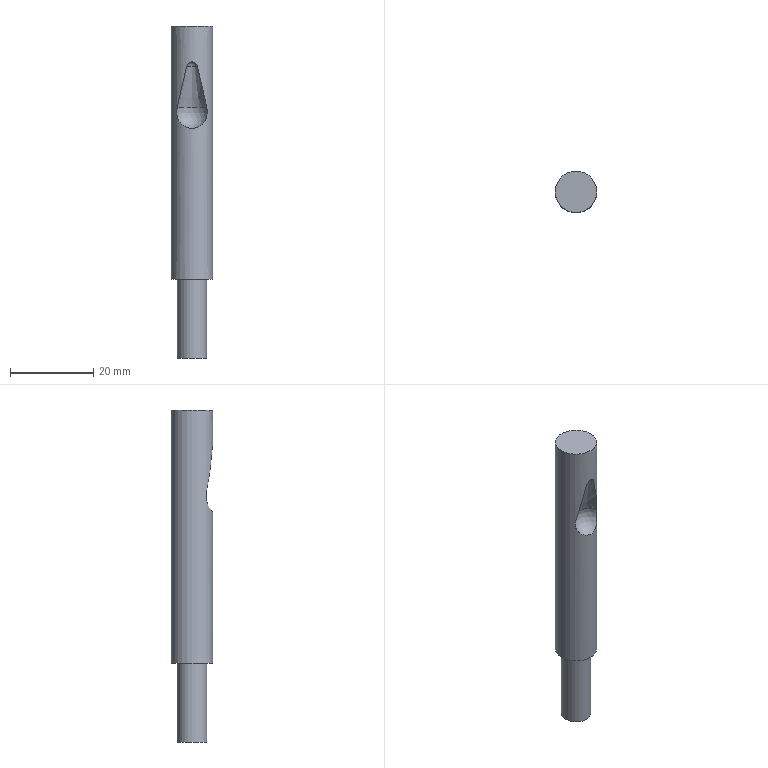Part | NX | features solid 2 | 1 solid | 8 faces | volume 5366 mm3 | plane 3 | cylinder 2 | sphere 2 | cone 1 | commonest cylinder face diameters 7.1 x1 10 x1
STEP:
#1=CARTESIAN_POINT('',(-337.549,205.711,111.333));
#2=VERTEX_POINT('',#1);
#3=CARTESIAN_POINT('',(-335.258,204.378,121.333));
#4=VERTEX_POINT('',#3);
#5=CARTESIAN_POINT('',(-337.549,205.711,111.333));
#6=CARTESIAN_POINT('',(-336.897,205.046,114.658));
#7=CARTESIAN_POINT('',(-336.099,204.6,117.992));
#8=CARTESIAN_POINT('',(-335.258,204.378,121.333));
#9=B_SPLINE_CURVE_WITH_KNOTS('',3,(#5,#6,#7,#8),.UNSPECIFIED.,.F.,.F.,(4,4),(0.000000207,0.01035),.UNSPECIFIED.);
#10=EDGE_CURVE('',#2,#4,#9,.T.);
#11=ORIENTED_EDGE('',*,*,#10,.T.);
#12=CARTESIAN_POINT('',(-332.698,204.378,121.333));
#13=VERTEX_POINT('',#12);
#14=CARTESIAN_POINT('',(-335.258,204.378,121.333));
#15=CARTESIAN_POINT('',(-335.114,204.339,121.906));
#16=CARTESIAN_POINT('',(-333.98,204.083,122.76));
#17=CARTESIAN_POINT('',(-332.842,204.339,121.906));
#18=CARTESIAN_POINT('',(-332.698,204.378,121.333));
#19=B_SPLINE_CURVE_WITH_KNOTS('',3,(#14,#15,#16,#17,#18),.UNSPECIFIED.,.F.,.F.,(4,1,4),(0.000000204,0.001751,0.003502),.UNSPECIFIED.);
#20=EDGE_CURVE('',#4,#13,#19,.T.);
#21=ORIENTED_EDGE('',*,*,#20,.T.);
#22=CARTESIAN_POINT('',(-330.407,205.711,111.333));
#23=VERTEX_POINT('',#22);
#24=CARTESIAN_POINT('',(-332.698,204.378,121.333));
#25=CARTESIAN_POINT('',(-331.856,204.6,117.991));
#26=CARTESIAN_POINT('',(-331.059,205.046,114.66));
#27=CARTESIAN_POINT('',(-330.407,205.711,111.333));
#28=B_SPLINE_CURVE_WITH_KNOTS('',3,(#24,#25,#26,#27),.UNSPECIFIED.,.F.,.F.,(4,4),(0.000000207,0.01036),.UNSPECIFIED.);
#29=EDGE_CURVE('',#13,#23,#28,.T.);
#30=ORIENTED_EDGE('',*,*,#29,.T.);
#31=CARTESIAN_POINT('',(-330.407,205.711,111.333));
#32=CARTESIAN_POINT('',(-330.29,205.83,110.737));
#33=CARTESIAN_POINT('',(-330.271,205.852,109.48));
#34=CARTESIAN_POINT('',(-330.868,205.236,107.792));
#35=CARTESIAN_POINT('',(-332.143,204.456,106.625));
#36=CARTESIAN_POINT('',(-333.967,204.089,106.188));
#37=CARTESIAN_POINT('',(-335.81,204.453,106.621));
#38=CARTESIAN_POINT('',(-337.087,205.236,107.792));
#39=CARTESIAN_POINT('',(-337.684,205.851,109.477));
#40=CARTESIAN_POINT('',(-337.666,205.83,110.737));
#41=CARTESIAN_POINT('',(-337.549,205.711,111.333));
#42=B_SPLINE_CURVE_WITH_KNOTS('',3,(#31,#32,#33,#34,#35,#36,#37,#38,#39,#40,#41),.UNSPECIFIED.,.F.,.F.,(4,1,1,1,1,1,1,1,4),(0.000000205,0.001831,0.003662,0.005493,0.007324,0.009155,0.01099,0.01282,0.01465),.UNSPECIFIED.);
#43=EDGE_CURVE('',#23,#2,#42,.T.);
#44=ORIENTED_EDGE('',*,*,#43,.T.);
#45=EDGE_LOOP('',(#11,#21,#30,#44));
#46=FACE_BOUND('',#45,.T.);
#47=CARTESIAN_POINT('',(-338.978,209.211,131.));
#48=VERTEX_POINT('',#47);
#49=CARTESIAN_POINT('',(-333.978,209.211,131.));
#50=DIRECTION('',(0.,0.,1.));
#51=DIRECTION('',(-1.,0.,0.));
#52=AXIS2_PLACEMENT_3D('',#49,#50,#51);
#53=CIRCLE('',#52,5.);
#54=EDGE_CURVE('',#48,#48,#53,.T.);
#55=ORIENTED_EDGE('',*,*,#54,.F.);
#56=EDGE_LOOP('',(#55));
#57=FACE_BOUND('',#56,.T.);
#58=CARTESIAN_POINT('',(-338.978,209.211,70.));
#59=VERTEX_POINT('',#58);
#60=CARTESIAN_POINT('',(-333.978,209.211,70.));
#61=DIRECTION('',(0.,0.,1.));
#62=DIRECTION('',(-1.,0.,0.));
#63=AXIS2_PLACEMENT_3D('',#60,#61,#62);
#64=CIRCLE('',#63,5.);
#65=EDGE_CURVE('',#59,#59,#64,.T.);
#66=ORIENTED_EDGE('',*,*,#65,.T.);
#67=EDGE_LOOP('',(#66));
#68=FACE_BOUND('',#67,.T.);
#69=CARTESIAN_POINT('',(-333.978,209.211,131.));
#70=DIRECTION('',(0.,0.,-1.));
#71=DIRECTION('',(1.,0.,0.));
#72=AXIS2_PLACEMENT_3D('',#69,#70,#71);
#73=CYLINDRICAL_SURFACE('',#72,5.);
#74=ADVANCED_FACE('',(#46,#57,#68),#73,.T.);
#75=ORIENTED_EDGE('',*,*,#54,.T.);
#76=EDGE_LOOP('',(#75));
#77=FACE_BOUND('',#76,.T.);
#78=CARTESIAN_POINT('',(-333.978,209.211,131.));
#79=DIRECTION('',(0.,0.,1.));
#80=DIRECTION('',(-1.,0.,0.));
#81=AXIS2_PLACEMENT_3D('',#78,#79,#80);
#82=PLANE('',#81);
#83=ADVANCED_FACE('',(#77),#82,.T.);
#84=CARTESIAN_POINT('',(-337.528,209.211,70.));
#85=VERTEX_POINT('',#84);
#86=CARTESIAN_POINT('',(-333.978,209.211,70.));
#87=DIRECTION('',(0.,0.,1.));
#88=DIRECTION('',(-1.,0.,0.));
#89=AXIS2_PLACEMENT_3D('',#86,#87,#88);
#90=CIRCLE('',#89,3.55);
#91=EDGE_CURVE('',#85,#85,#90,.T.);
#92=ORIENTED_EDGE('',*,*,#91,.T.);
#93=EDGE_LOOP('',(#92));
#94=FACE_BOUND('',#93,.T.);
#95=ORIENTED_EDGE('',*,*,#65,.F.);
#96=EDGE_LOOP('',(#95));
#97=FACE_BOUND('',#96,.T.);
#98=CARTESIAN_POINT('',(-333.978,209.211,70.));
#99=DIRECTION('',(0.,0.,1.));
#100=DIRECTION('',(-1.,0.,0.));
#101=AXIS2_PLACEMENT_3D('',#98,#99,#100);
#102=PLANE('',#101);
#103=ADVANCED_FACE('',(#94,#97),#102,.F.);
#104=CARTESIAN_POINT('',(-337.528,209.211,51.));
#105=VERTEX_POINT('',#104);
#106=CARTESIAN_POINT('',(-333.978,209.211,51.));
#107=DIRECTION('',(0.,0.,1.));
#108=DIRECTION('',(-1.,0.,0.));
#109=AXIS2_PLACEMENT_3D('',#106,#107,#108);
#110=CIRCLE('',#109,3.55);
#111=EDGE_CURVE('',#105,#105,#110,.T.);
#112=ORIENTED_EDGE('',*,*,#111,.T.);
#113=EDGE_LOOP('',(#112));
#114=FACE_BOUND('',#113,.T.);
#115=ORIENTED_EDGE('',*,*,#91,.F.);
#116=EDGE_LOOP('',(#115));
#117=FACE_BOUND('',#116,.T.);
#118=CARTESIAN_POINT('',(-333.978,209.211,51.));
#119=DIRECTION('',(0.,0.,1.));
#120=DIRECTION('',(-1.,0.,0.));
#121=AXIS2_PLACEMENT_3D('',#118,#119,#120);
#122=CYLINDRICAL_SURFACE('',#121,3.55);
#123=ADVANCED_FACE('',(#114,#117),#122,.T.);
#124=ORIENTED_EDGE('',*,*,#111,.F.);
#125=EDGE_LOOP('',(#124));
#126=FACE_BOUND('',#125,.T.);
#127=CARTESIAN_POINT('',(-333.978,209.211,51.));
#128=DIRECTION('',(0.,0.,1.));
#129=DIRECTION('',(-1.,0.,0.));
#130=AXIS2_PLACEMENT_3D('',#127,#128,#129);
#131=PLANE('',#130);
#132=ADVANCED_FACE('',(#126),#131,.F.);
#133=CARTESIAN_POINT('',(-333.978,204.211,111.333));
#134=DIRECTION('',(0.,0.,-1.));
#135=DIRECTION('',(1.,0.,0.));
#136=AXIS2_PLACEMENT_3D('',#133,#134,#135);
#137=CIRCLE('',#136,3.873);
#138=EDGE_CURVE('',#2,#23,#137,.T.);
#139=ORIENTED_EDGE('',*,*,#138,.F.);
#140=ORIENTED_EDGE('',*,*,#43,.F.);
#141=EDGE_LOOP('',(#139,#140));
#142=FACE_BOUND('',#141,.T.);
#143=CARTESIAN_POINT('',(-333.978,204.211,110.333));
#144=DIRECTION('',(0.,0.,-1.));
#145=DIRECTION('',(1.,0.,0.));
#146=AXIS2_PLACEMENT_3D('',#143,#144,#145);
#147=SPHERICAL_SURFACE('',#146,4.);
#148=ADVANCED_FACE('',(#142),#147,.F.);
#149=CARTESIAN_POINT('',(-333.978,204.211,121.333));
#150=DIRECTION('',(0.,0.,-1.));
#151=DIRECTION('',(1.,0.,0.));
#152=AXIS2_PLACEMENT_3D('',#149,#150,#151);
#153=CIRCLE('',#152,1.291);
#154=EDGE_CURVE('',#4,#13,#153,.T.);
#155=ORIENTED_EDGE('',*,*,#154,.F.);
#156=ORIENTED_EDGE('',*,*,#10,.F.);
#157=ORIENTED_EDGE('',*,*,#138,.T.);
#158=ORIENTED_EDGE('',*,*,#29,.F.);
#159=EDGE_LOOP('',(#155,#156,#157,#158));
#160=FACE_BOUND('',#159,.T.);
#161=CARTESIAN_POINT('',(-333.978,204.211,111.333));
#162=DIRECTION('',(0.,0.,-1.));
#163=DIRECTION('',(1.,0.,0.));
#164=AXIS2_PLACEMENT_3D('',#161,#162,#163);
#165=CONICAL_SURFACE('',#164,3.873,0.2527);
#166=ADVANCED_FACE('',(#160),#165,.F.);
#167=ORIENTED_EDGE('',*,*,#154,.T.);
#168=ORIENTED_EDGE('',*,*,#20,.F.);
#169=EDGE_LOOP('',(#167,#168));
#170=FACE_BOUND('',#169,.T.);
#171=CARTESIAN_POINT('',(-333.978,204.211,121.));
#172=DIRECTION('',(0.,0.,-1.));
#173=DIRECTION('',(-1.,0.,0.));
#174=AXIS2_PLACEMENT_3D('',#171,#172,#173);
#175=SPHERICAL_SURFACE('',#174,1.333);
#176=ADVANCED_FACE('',(#170),#175,.F.);
#177=CLOSED_SHELL('',(#74,#83,#103,#123,#132,#148,#166,#176));
#178=MANIFOLD_SOLID_BREP('',#177);
#179=(LENGTH_UNIT()NAMED_UNIT(*)SI_UNIT(.MILLI.,.METRE.));
#180=UNCERTAINTY_MEASURE_WITH_UNIT(LENGTH_MEASURE(0.0508),#179,'','');
#181=(NAMED_UNIT(*)PLANE_ANGLE_UNIT()SI_UNIT($,.RADIAN.));
#182=(NAMED_UNIT(*)SI_UNIT($,.STERADIAN.)SOLID_ANGLE_UNIT());
#183=(GEOMETRIC_REPRESENTATION_CONTEXT(3)GLOBAL_UNCERTAINTY_ASSIGNED_CONTEXT((#180))GLOBAL_UNIT_ASSIGNED_CONTEXT((#179,#181,#182))REPRESENTATION_CONTEXT('',''));
#184=ADVANCED_BREP_SHAPE_REPRESENTATION('',(#178),#183);